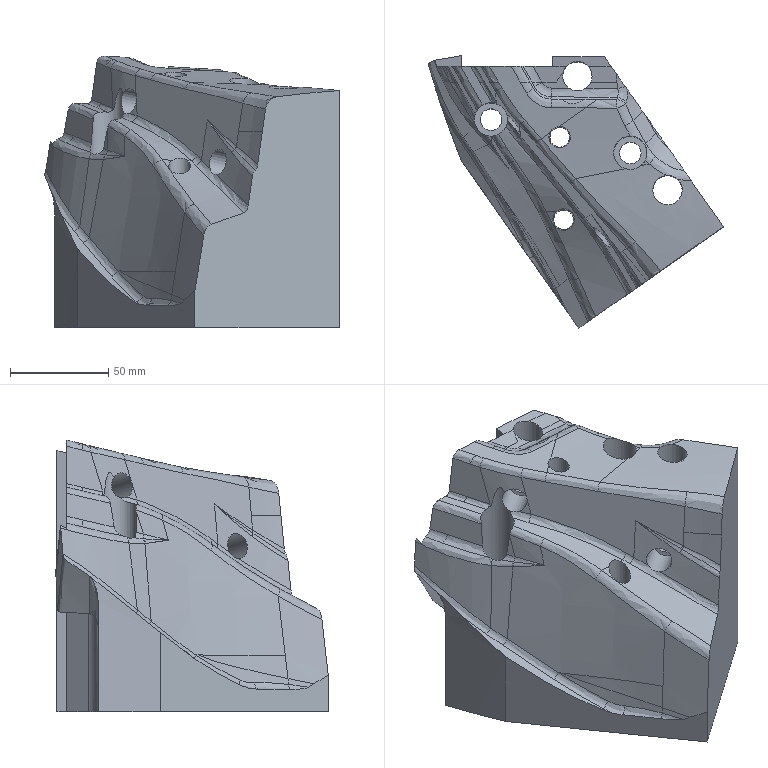Part | NX | features solid 2 | 1 solid | 137 faces | box 150.321 x 138.916 x 138.635 mm | volume 1040993 mm3 | spline 104 | plane 17 | cylinder 16 | commonest cylinder face diameters 10 x4 11 x4 9 x2 13 x2 15 x2 17 x2